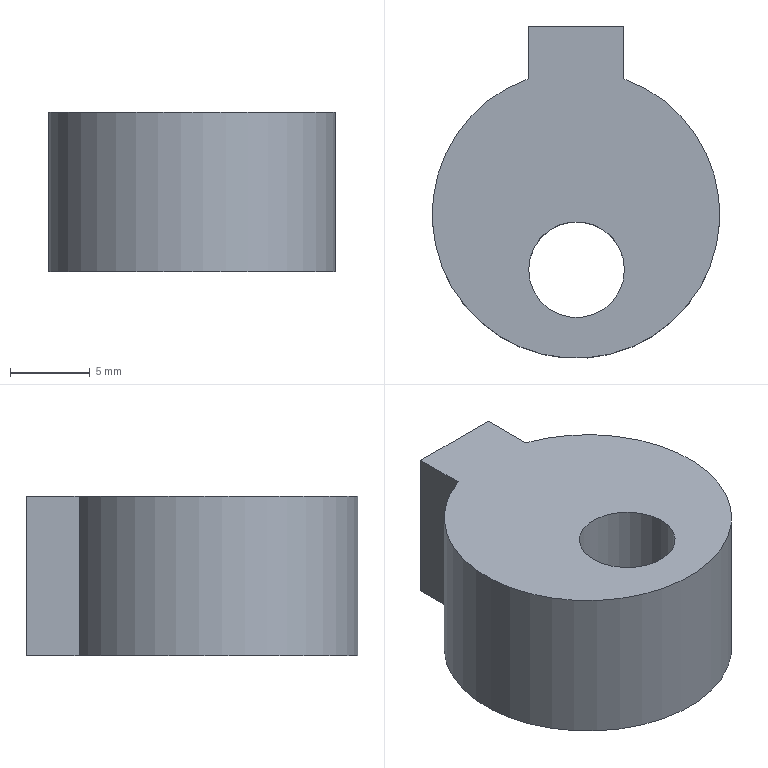Part | NX | 1 solid | 7 faces | box 18 x 20.8 x 10 mm | volume 2440 mm3 | plane 5 | cylinder 2 | commonest cylinder face diameters 6 x1 18 x1
STEP:
#1=CARTESIAN_POINT('',(-2.965,-3.453,18.8));
#2=VERTEX_POINT('',#1);
#3=CARTESIAN_POINT('',(0.03502,-3.453,18.8));
#4=DIRECTION('',(0.,0.,-1.));
#5=DIRECTION('',(-1.,0.,0.));
#6=AXIS2_PLACEMENT_3D('',#3,#4,#5);
#7=CIRCLE('',#6,3.);
#8=EDGE_CURVE('',#2,#2,#7,.T.);
#9=ORIENTED_EDGE('',*,*,#8,.T.);
#10=EDGE_LOOP('',(#9));
#11=FACE_BOUND('',#10,.T.);
#12=CARTESIAN_POINT('',(3.,11.8,18.8));
#13=VERTEX_POINT('',#12);
#14=CARTESIAN_POINT('',(-3.,11.8,18.8));
#15=VERTEX_POINT('',#14);
#16=CARTESIAN_POINT('',(3.,11.8,18.8));
#17=DIRECTION('',(-1.,0.,0.));
#18=VECTOR('',#17,1000.);
#19=LINE('',#16,#18);
#20=EDGE_CURVE('',#13,#15,#19,.T.);
#21=ORIENTED_EDGE('',*,*,#20,.T.);
#22=CARTESIAN_POINT('',(-3.,8.485,18.8));
#23=VERTEX_POINT('',#22);
#24=CARTESIAN_POINT('',(-3.,11.8,18.8));
#25=DIRECTION('',(0.,-1.,0.));
#26=VECTOR('',#25,1000.);
#27=LINE('',#24,#26);
#28=EDGE_CURVE('',#15,#23,#27,.T.);
#29=ORIENTED_EDGE('',*,*,#28,.T.);
#30=CARTESIAN_POINT('',(3.,8.485,18.8));
#31=VERTEX_POINT('',#30);
#32=CARTESIAN_POINT('',(0.,0.,18.8));
#33=DIRECTION('',(0.,0.,1.));
#34=DIRECTION('',(1.,0.,0.));
#35=AXIS2_PLACEMENT_3D('',#32,#33,#34);
#36=CIRCLE('',#35,9.);
#37=EDGE_CURVE('',#23,#31,#36,.T.);
#38=ORIENTED_EDGE('',*,*,#37,.T.);
#39=CARTESIAN_POINT('',(3.,8.485,18.8));
#40=DIRECTION('',(0.,1.,0.));
#41=VECTOR('',#40,1000.);
#42=LINE('',#39,#41);
#43=EDGE_CURVE('',#31,#13,#42,.T.);
#44=ORIENTED_EDGE('',*,*,#43,.T.);
#45=EDGE_LOOP('',(#21,#29,#38,#44));
#46=FACE_BOUND('',#45,.T.);
#47=CARTESIAN_POINT('',(0.,0.,18.8));
#48=DIRECTION('',(0.,0.,1.));
#49=DIRECTION('',(1.,0.,0.));
#50=AXIS2_PLACEMENT_3D('',#47,#48,#49);
#51=PLANE('',#50);
#52=ADVANCED_FACE('',(#11,#46),#51,.T.);
#53=CARTESIAN_POINT('',(3.,8.485,8.8));
#54=VERTEX_POINT('',#53);
#55=CARTESIAN_POINT('',(3.,8.485,21.8));
#56=DIRECTION('',(0.,0.,-1.));
#57=VECTOR('',#56,1000.);
#58=LINE('',#55,#57);
#59=EDGE_CURVE('',#31,#54,#58,.T.);
#60=ORIENTED_EDGE('',*,*,#59,.T.);
#61=CARTESIAN_POINT('',(3.,11.8,8.8));
#62=VERTEX_POINT('',#61);
#63=CARTESIAN_POINT('',(3.,11.8,8.8));
#64=DIRECTION('',(0.,-1.,0.));
#65=VECTOR('',#64,1000.);
#66=LINE('',#63,#65);
#67=EDGE_CURVE('',#62,#54,#66,.T.);
#68=ORIENTED_EDGE('',*,*,#67,.F.);
#69=CARTESIAN_POINT('',(3.,11.8,21.8));
#70=DIRECTION('',(0.,0.,-1.));
#71=VECTOR('',#70,1000.);
#72=LINE('',#69,#71);
#73=EDGE_CURVE('',#13,#62,#72,.T.);
#74=ORIENTED_EDGE('',*,*,#73,.F.);
#75=ORIENTED_EDGE('',*,*,#43,.F.);
#76=EDGE_LOOP('',(#60,#68,#74,#75));
#77=FACE_BOUND('',#76,.T.);
#78=CARTESIAN_POINT('',(3.,8.485,21.8));
#79=DIRECTION('',(-1.,0.,0.));
#80=DIRECTION('',(0.,-1.,0.));
#81=AXIS2_PLACEMENT_3D('',#78,#79,#80);
#82=PLANE('',#81);
#83=ADVANCED_FACE('',(#77),#82,.F.);
#84=CARTESIAN_POINT('',(-3.,8.485,8.8));
#85=VERTEX_POINT('',#84);
#86=CARTESIAN_POINT('',(-3.,8.485,21.8));
#87=DIRECTION('',(0.,0.,-1.));
#88=VECTOR('',#87,1000.);
#89=LINE('',#86,#88);
#90=EDGE_CURVE('',#23,#85,#89,.T.);
#91=ORIENTED_EDGE('',*,*,#90,.T.);
#92=CARTESIAN_POINT('',(0.,0.,8.8));
#93=DIRECTION('',(0.,0.,-1.));
#94=DIRECTION('',(1.,0.,0.));
#95=AXIS2_PLACEMENT_3D('',#92,#93,#94);
#96=CIRCLE('',#95,9.);
#97=EDGE_CURVE('',#54,#85,#96,.T.);
#98=ORIENTED_EDGE('',*,*,#97,.F.);
#99=ORIENTED_EDGE('',*,*,#59,.F.);
#100=ORIENTED_EDGE('',*,*,#37,.F.);
#101=EDGE_LOOP('',(#91,#98,#99,#100));
#102=FACE_BOUND('',#101,.T.);
#103=CARTESIAN_POINT('',(0.,0.,21.8));
#104=DIRECTION('',(0.,0.,-1.));
#105=DIRECTION('',(-1.,0.,0.));
#106=AXIS2_PLACEMENT_3D('',#103,#104,#105);
#107=CYLINDRICAL_SURFACE('',#106,9.);
#108=ADVANCED_FACE('',(#102),#107,.T.);
#109=CARTESIAN_POINT('',(-3.,11.8,8.8));
#110=VERTEX_POINT('',#109);
#111=CARTESIAN_POINT('',(-3.,11.8,21.8));
#112=DIRECTION('',(0.,0.,-1.));
#113=VECTOR('',#112,1000.);
#114=LINE('',#111,#113);
#115=EDGE_CURVE('',#15,#110,#114,.T.);
#116=ORIENTED_EDGE('',*,*,#115,.T.);
#117=CARTESIAN_POINT('',(-3.,8.485,8.8));
#118=DIRECTION('',(0.,1.,0.));
#119=VECTOR('',#118,1000.);
#120=LINE('',#117,#119);
#121=EDGE_CURVE('',#85,#110,#120,.T.);
#122=ORIENTED_EDGE('',*,*,#121,.F.);
#123=ORIENTED_EDGE('',*,*,#90,.F.);
#124=ORIENTED_EDGE('',*,*,#28,.F.);
#125=EDGE_LOOP('',(#116,#122,#123,#124));
#126=FACE_BOUND('',#125,.T.);
#127=CARTESIAN_POINT('',(-3.,11.8,21.8));
#128=DIRECTION('',(1.,0.,0.));
#129=DIRECTION('',(0.,1.,0.));
#130=AXIS2_PLACEMENT_3D('',#127,#128,#129);
#131=PLANE('',#130);
#132=ADVANCED_FACE('',(#126),#131,.F.);
#133=ORIENTED_EDGE('',*,*,#73,.T.);
#134=CARTESIAN_POINT('',(-3.,11.8,8.8));
#135=DIRECTION('',(1.,0.,0.));
#136=VECTOR('',#135,1000.);
#137=LINE('',#134,#136);
#138=EDGE_CURVE('',#110,#62,#137,.T.);
#139=ORIENTED_EDGE('',*,*,#138,.F.);
#140=ORIENTED_EDGE('',*,*,#115,.F.);
#141=ORIENTED_EDGE('',*,*,#20,.F.);
#142=EDGE_LOOP('',(#133,#139,#140,#141));
#143=FACE_BOUND('',#142,.T.);
#144=CARTESIAN_POINT('',(3.,11.8,21.8));
#145=DIRECTION('',(0.,-1.,0.));
#146=DIRECTION('',(0.,0.,-1.));
#147=AXIS2_PLACEMENT_3D('',#144,#145,#146);
#148=PLANE('',#147);
#149=ADVANCED_FACE('',(#143),#148,.F.);
#150=CARTESIAN_POINT('',(3.035,-3.453,8.8));
#151=VERTEX_POINT('',#150);
#152=CARTESIAN_POINT('',(0.03502,-3.453,8.8));
#153=DIRECTION('',(0.,0.,1.));
#154=DIRECTION('',(1.,0.,0.));
#155=AXIS2_PLACEMENT_3D('',#152,#153,#154);
#156=CIRCLE('',#155,3.);
#157=EDGE_CURVE('',#151,#151,#156,.T.);
#158=ORIENTED_EDGE('',*,*,#157,.T.);
#159=EDGE_LOOP('',(#158));
#160=FACE_BOUND('',#159,.T.);
#161=ORIENTED_EDGE('',*,*,#67,.T.);
#162=ORIENTED_EDGE('',*,*,#97,.T.);
#163=ORIENTED_EDGE('',*,*,#121,.T.);
#164=ORIENTED_EDGE('',*,*,#138,.T.);
#165=EDGE_LOOP('',(#161,#162,#163,#164));
#166=FACE_BOUND('',#165,.T.);
#167=CARTESIAN_POINT('',(0.,0.,8.8));
#168=DIRECTION('',(0.,0.,1.));
#169=DIRECTION('',(1.,0.,0.));
#170=AXIS2_PLACEMENT_3D('',#167,#168,#169);
#171=PLANE('',#170);
#172=ADVANCED_FACE('',(#160,#166),#171,.F.);
#173=ORIENTED_EDGE('',*,*,#8,.F.);
#174=EDGE_LOOP('',(#173));
#175=FACE_BOUND('',#174,.T.);
#176=ORIENTED_EDGE('',*,*,#157,.F.);
#177=EDGE_LOOP('',(#176));
#178=FACE_BOUND('',#177,.T.);
#179=CARTESIAN_POINT('',(0.03502,-3.453,18.8));
#180=DIRECTION('',(0.,0.,-1.));
#181=DIRECTION('',(-1.,0.,0.));
#182=AXIS2_PLACEMENT_3D('',#179,#180,#181);
#183=CYLINDRICAL_SURFACE('',#182,3.);
#184=ADVANCED_FACE('',(#175,#178),#183,.F.);
#185=CLOSED_SHELL('',(#52,#83,#108,#132,#149,#172,#184));
#186=MANIFOLD_SOLID_BREP('',#185);
#187=(LENGTH_UNIT()NAMED_UNIT(*)SI_UNIT(.MILLI.,.METRE.));
#188=UNCERTAINTY_MEASURE_WITH_UNIT(LENGTH_MEASURE(0.00001),#187,'','');
#189=(NAMED_UNIT(*)PLANE_ANGLE_UNIT()SI_UNIT($,.RADIAN.));
#190=(NAMED_UNIT(*)SI_UNIT($,.STERADIAN.)SOLID_ANGLE_UNIT());
#191=(GEOMETRIC_REPRESENTATION_CONTEXT(3)GLOBAL_UNCERTAINTY_ASSIGNED_CONTEXT((#188))GLOBAL_UNIT_ASSIGNED_CONTEXT((#187,#189,#190))REPRESENTATION_CONTEXT('',''));
#192=ADVANCED_BREP_SHAPE_REPRESENTATION('',(#186),#191);